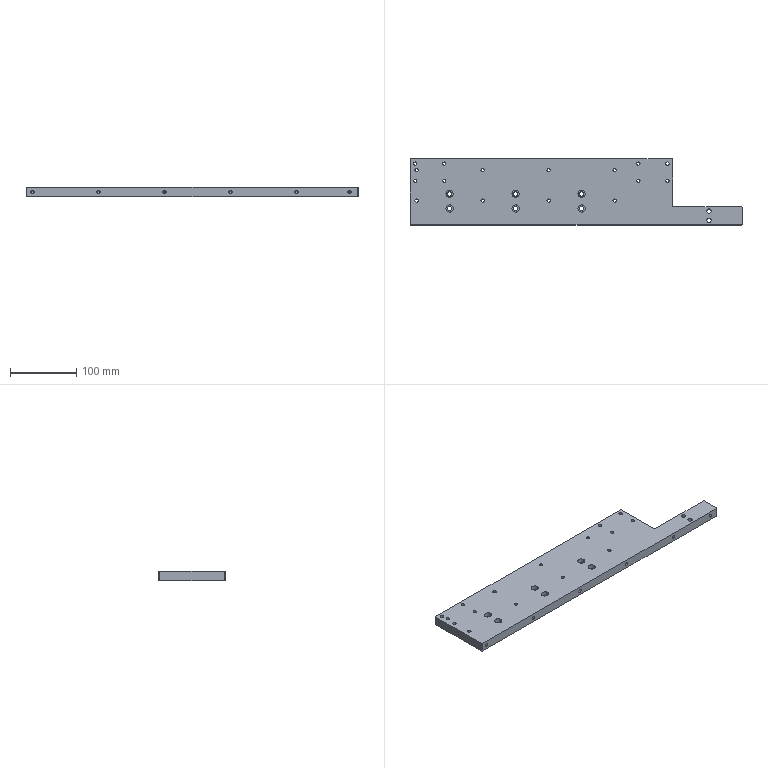Part | SolidWorks | features HoleWzd 5, Chamfer 1, Extrusion 1, ICE 1 | 1 solid | 103 faces | box 503 x 100 x 14 mm | volume 585787 mm3 | cylinder 72 | plane 19 | cone 12 | commonest cylinder face diameters 5 x44 6.6 x16 11 x12